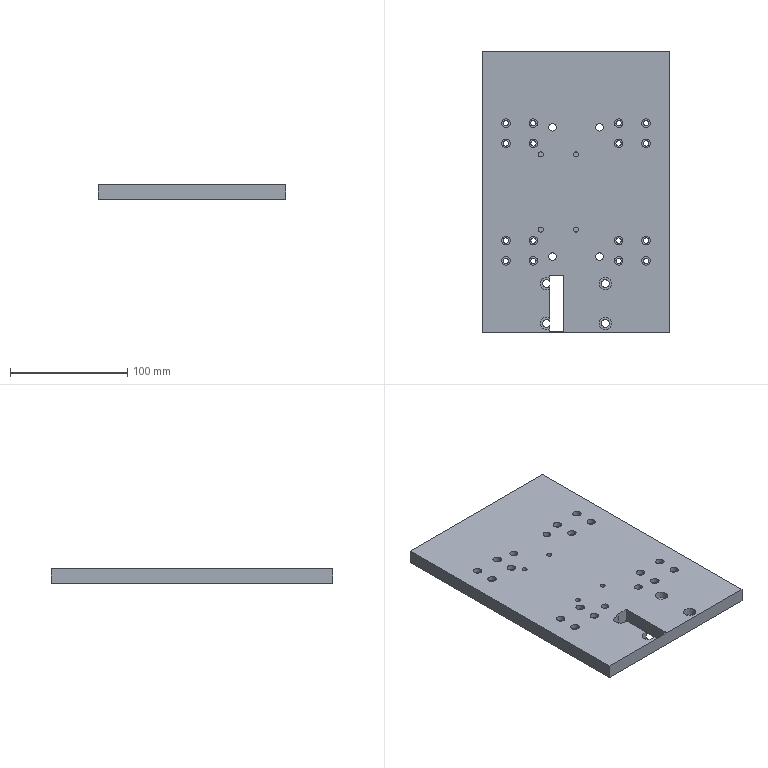Part | SolidWorks | features BaseBody 1 | 1 solid | 128 faces | box 160 x 240 x 12 mm | volume 444338 mm3 | cylinder 92 | plane 36 | commonest cylinder face diameters 4.5 x32 7.2 x32 6.5 x14 4.3 x8 10.6 x6